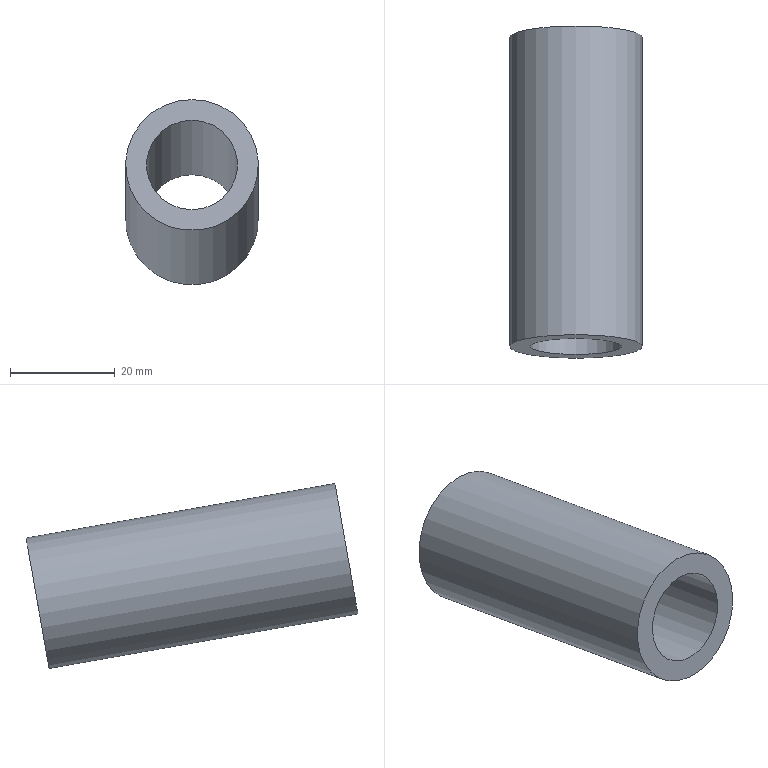Part | NX | features solid 2 | 1 solid | 4 faces | box 25.4 x 63.499 x 35.433 mm | volume 16135 mm3 | cylinder 2 | plane 2 | commonest cylinder face diameters 17.4 x1 25.4 x1
STEP:
#1=CARTESIAN_POINT('',(776.5,-783.217,18.524));
#2=VERTEX_POINT('',#1);
#3=CARTESIAN_POINT('',(776.5,-784.728,9.956));
#4=DIRECTION('',(0.,0.9848,-0.1736));
#5=DIRECTION('',(0.,0.1736,0.9848));
#6=AXIS2_PLACEMENT_3D('',#3,#4,#5);
#7=CIRCLE('',#6,8.7);
#8=EDGE_CURVE('',#2,#2,#7,.F.);
#9=ORIENTED_EDGE('',*,*,#8,.T.);
#10=EDGE_LOOP('',(#9));
#11=FACE_BOUND('',#10,.T.);
#12=CARTESIAN_POINT('',(776.5,-724.129,8.105));
#13=VERTEX_POINT('',#12);
#14=CARTESIAN_POINT('',(776.5,-725.639,-0.4626));
#15=DIRECTION('',(0.,0.9848,-0.1736));
#16=DIRECTION('',(0.,0.1736,0.9848));
#17=AXIS2_PLACEMENT_3D('',#14,#15,#16);
#18=CIRCLE('',#17,8.7);
#19=EDGE_CURVE('',#13,#13,#18,.F.);
#20=ORIENTED_EDGE('',*,*,#19,.F.);
#21=EDGE_LOOP('',(#20));
#22=FACE_BOUND('',#21,.T.);
#23=CARTESIAN_POINT('',(776.5,-863.513,23.848));
#24=DIRECTION('',(0.,0.9848,-0.1736));
#25=DIRECTION('',(1.,0.,0.));
#26=AXIS2_PLACEMENT_3D('',#23,#24,#25);
#27=CYLINDRICAL_SURFACE('',#26,8.7);
#28=ADVANCED_FACE('',(#11,#22),#27,.F.);
#29=CARTESIAN_POINT('',(776.5,-782.523,22.463));
#30=VERTEX_POINT('',#29);
#31=CARTESIAN_POINT('',(776.5,-784.728,9.956));
#32=DIRECTION('',(0.,0.9848,-0.1736));
#33=DIRECTION('',(0.,0.1736,0.9848));
#34=AXIS2_PLACEMENT_3D('',#31,#32,#33);
#35=CIRCLE('',#34,12.7);
#36=EDGE_CURVE('',#30,#30,#35,.F.);
#37=ORIENTED_EDGE('',*,*,#36,.F.);
#38=EDGE_LOOP('',(#37));
#39=FACE_BOUND('',#38,.T.);
#40=CARTESIAN_POINT('',(776.5,-723.434,12.044));
#41=VERTEX_POINT('',#40);
#42=CARTESIAN_POINT('',(776.5,-725.639,-0.4626));
#43=DIRECTION('',(0.,0.9848,-0.1736));
#44=DIRECTION('',(0.,0.1736,0.9848));
#45=AXIS2_PLACEMENT_3D('',#42,#43,#44);
#46=CIRCLE('',#45,12.7);
#47=EDGE_CURVE('',#41,#41,#46,.F.);
#48=ORIENTED_EDGE('',*,*,#47,.T.);
#49=EDGE_LOOP('',(#48));
#50=FACE_BOUND('',#49,.T.);
#51=CARTESIAN_POINT('',(776.5,-863.513,23.848));
#52=DIRECTION('',(0.,0.9848,-0.1736));
#53=DIRECTION('',(1.,0.,0.));
#54=AXIS2_PLACEMENT_3D('',#51,#52,#53);
#55=CYLINDRICAL_SURFACE('',#54,12.7);
#56=ADVANCED_FACE('',(#39,#50),#55,.T.);
#57=ORIENTED_EDGE('',*,*,#8,.F.);
#58=EDGE_LOOP('',(#57));
#59=FACE_BOUND('',#58,.T.);
#60=ORIENTED_EDGE('',*,*,#36,.T.);
#61=EDGE_LOOP('',(#60));
#62=FACE_BOUND('',#61,.T.);
#63=CARTESIAN_POINT('',(776.5,-784.728,9.956));
#64=DIRECTION('',(0.,-0.9848,0.1736));
#65=DIRECTION('',(-1.,0.,0.));
#66=AXIS2_PLACEMENT_3D('',#63,#64,#65);
#67=PLANE('',#66);
#68=ADVANCED_FACE('',(#59,#62),#67,.T.);
#69=ORIENTED_EDGE('',*,*,#19,.T.);
#70=EDGE_LOOP('',(#69));
#71=FACE_BOUND('',#70,.T.);
#72=ORIENTED_EDGE('',*,*,#47,.F.);
#73=EDGE_LOOP('',(#72));
#74=FACE_BOUND('',#73,.T.);
#75=CARTESIAN_POINT('',(776.5,-725.639,-0.4626));
#76=DIRECTION('',(0.,-0.9848,0.1736));
#77=DIRECTION('',(-1.,0.,0.));
#78=AXIS2_PLACEMENT_3D('',#75,#76,#77);
#79=PLANE('',#78);
#80=ADVANCED_FACE('',(#71,#74),#79,.F.);
#81=CLOSED_SHELL('',(#28,#56,#68,#80));
#82=MANIFOLD_SOLID_BREP('',#81);
#83=(LENGTH_UNIT()NAMED_UNIT(*)SI_UNIT(.MILLI.,.METRE.));
#84=UNCERTAINTY_MEASURE_WITH_UNIT(LENGTH_MEASURE(0.00001),#83,'','');
#85=(NAMED_UNIT(*)PLANE_ANGLE_UNIT()SI_UNIT($,.RADIAN.));
#86=(NAMED_UNIT(*)SI_UNIT($,.STERADIAN.)SOLID_ANGLE_UNIT());
#87=(GEOMETRIC_REPRESENTATION_CONTEXT(3)GLOBAL_UNCERTAINTY_ASSIGNED_CONTEXT((#84))GLOBAL_UNIT_ASSIGNED_CONTEXT((#83,#85,#86))REPRESENTATION_CONTEXT('',''));
#88=ADVANCED_BREP_SHAPE_REPRESENTATION('',(#82),#87);